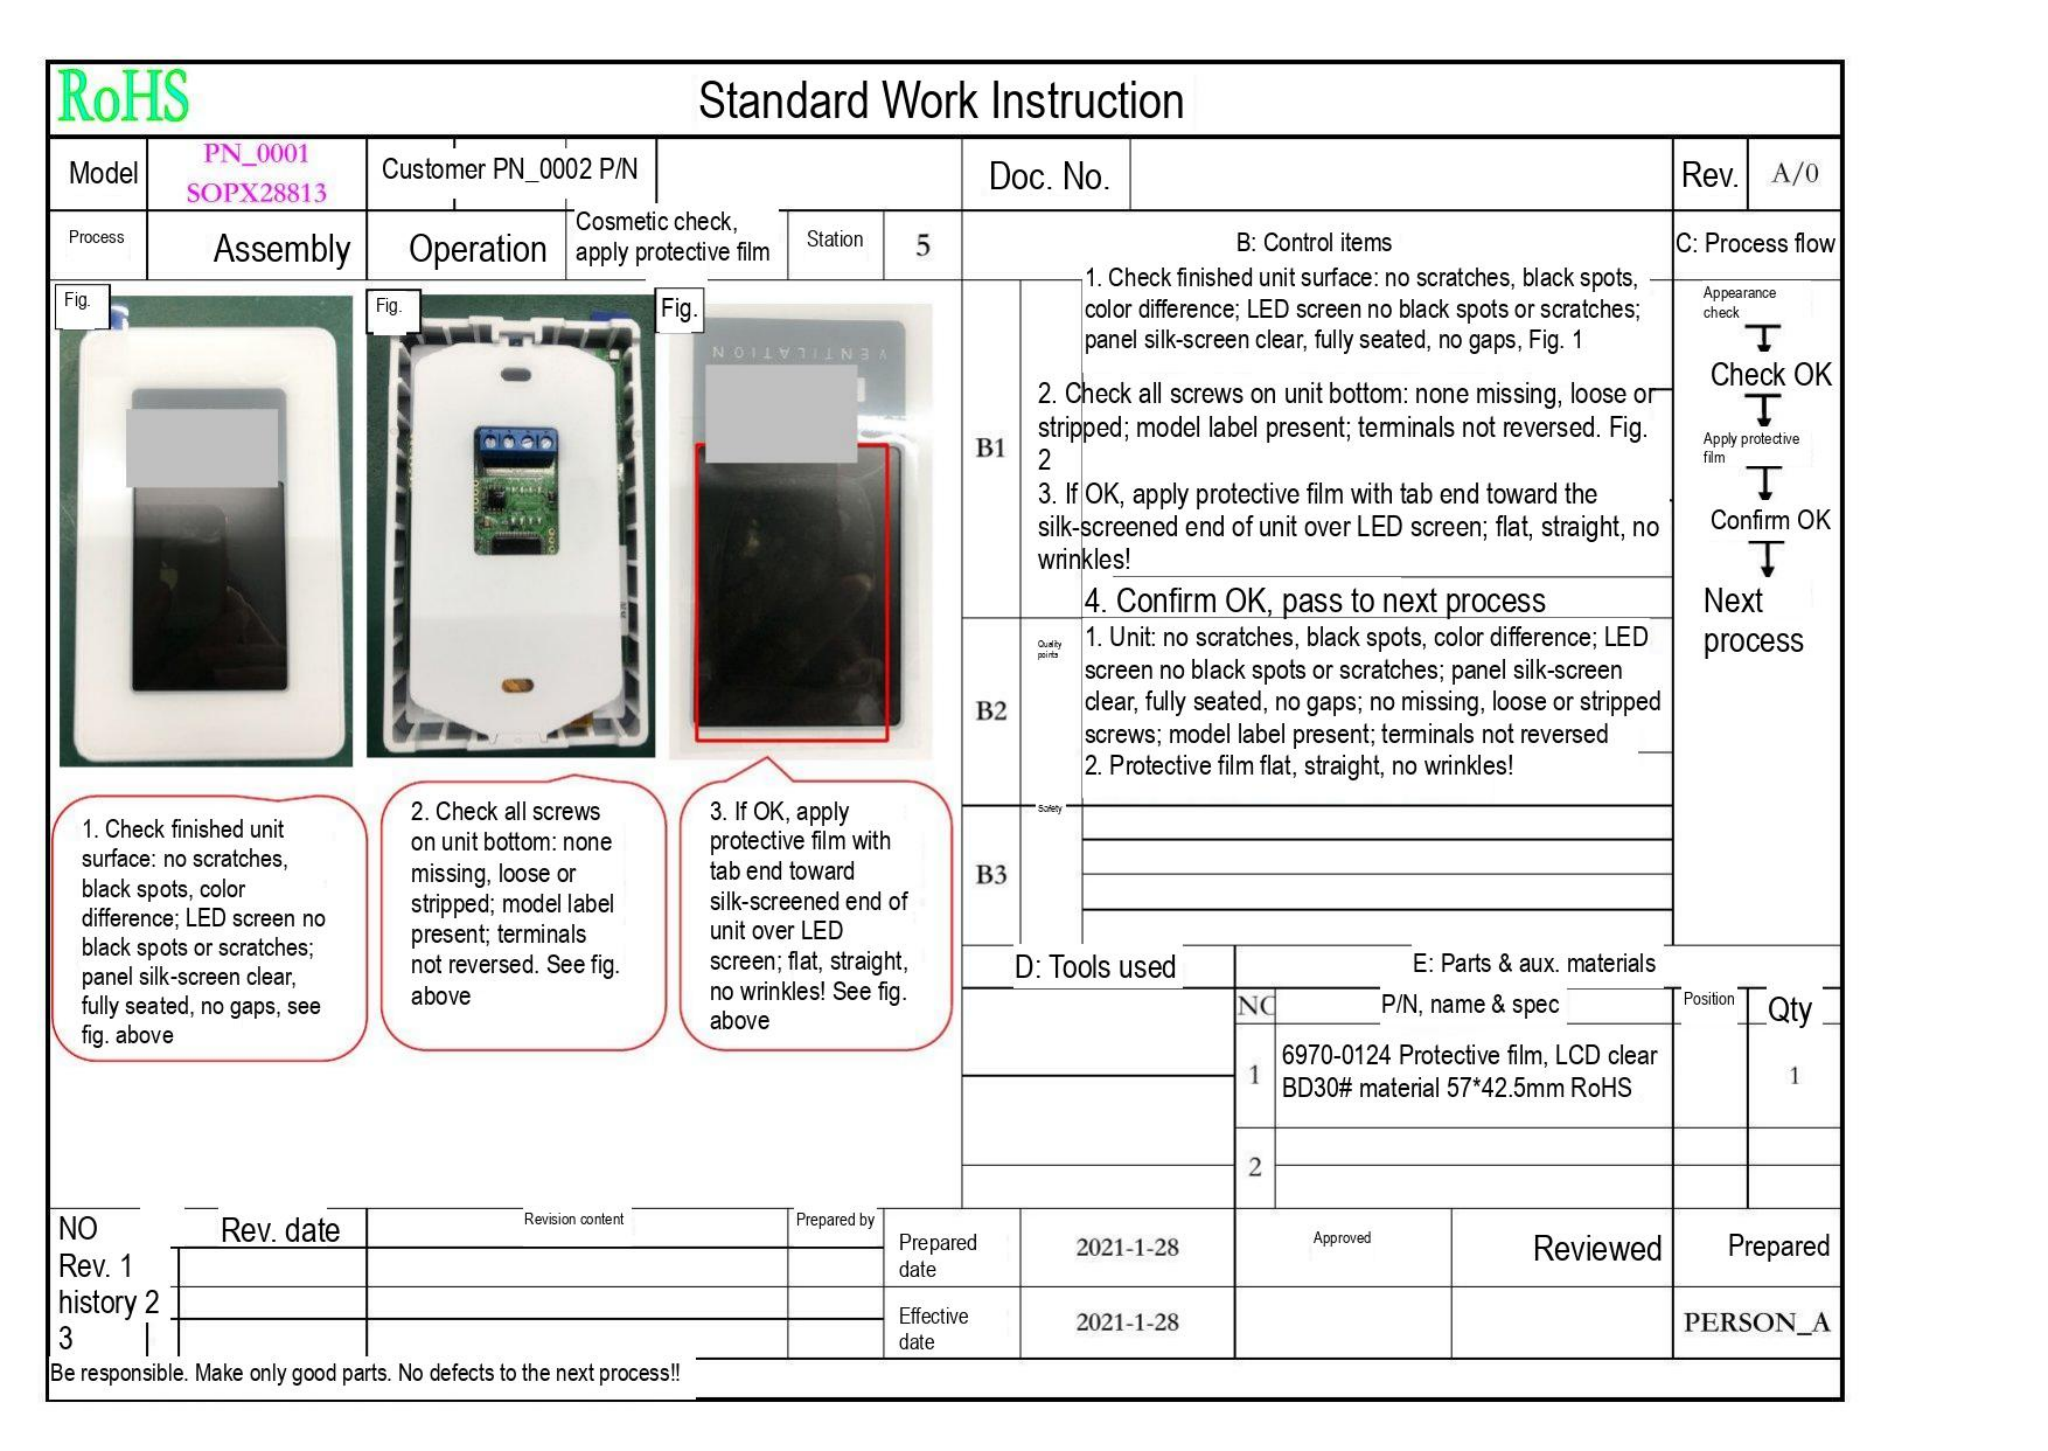RoHS

# Standard Work Instruction

| Model | PN_0001 SOPX28813 | Customer PN_0002 P/N | | Doc. No. | | Rev. | A/0 |
|---|---|---|---|---|---|---|---|
| Process | Assembly | Operation | Cosmetic check, apply protective film | Station | 5 | | |

Fig.

Fig.

Fig.

VENTILATION

1. Check finished unit surface: no scratches, black spots, color difference; LED screen no black spots or scratches; panel silk-screen clear, fully seated, no gaps, see fig. above

2. Check all screws on unit bottom: none missing, loose or stripped; model label present; terminals not reversed. See fig. above

3. If OK, apply protective film with tab end toward silk-screened end of unit over LED screen; flat, straight, no wrinkles! See fig. above

B: Control items

| | | |
|---|---|---|
| B1 | | 1. Check finished unit surface: no scratches, black spots, color difference; LED screen no black spots or scratches; panel silk-screen clear, fully seated, no gaps, Fig. 1<br>2. Check all screws on unit bottom: none missing, loose or stripped; model label present; terminals not reversed. Fig. 2<br>3. If OK, apply protective film with tab end toward the silk-screened end of unit over LED screen; flat, straight, no wrinkles!<br>4. Confirm OK, pass to next process |
| B2 | Quality points | 1. Unit: no scratches, black spots, color difference; LED screen no black spots or scratches; panel silk-screen clear, fully seated, no gaps; no missing, loose or stripped screws; model label present; terminals not reversed<br>2. Protective film flat, straight, no wrinkles! |
| B3 | Safety | |

C: Process flow

Appearance check
↓
Check OK
↓
Apply protective film
↓
Confirm OK
↓
Next process

D: Tools used

E: Parts & aux. materials

| NO | P/N, name & spec | Position | Qty |
|---|---|---|---|
| 1 | 6970-0124 Protective film, LCD clear BD30# material 57*42.5mm RoHS | | 1 |
| 2 | | | |

| NO | Rev. date | Revision content | Prepared by |
|---|---|---|---|
| Rev. 1 | | | |
| history 2 | | | |
| 3 | | | |

| | | Approved | Reviewed | Prepared |
|---|---|---|---|---|
| Prepared date | 2021-1-28 | | | |
| Effective date | 2021-1-28 | | | PERSON_A |

Be responsible. Make only good parts. No defects to the next process!!
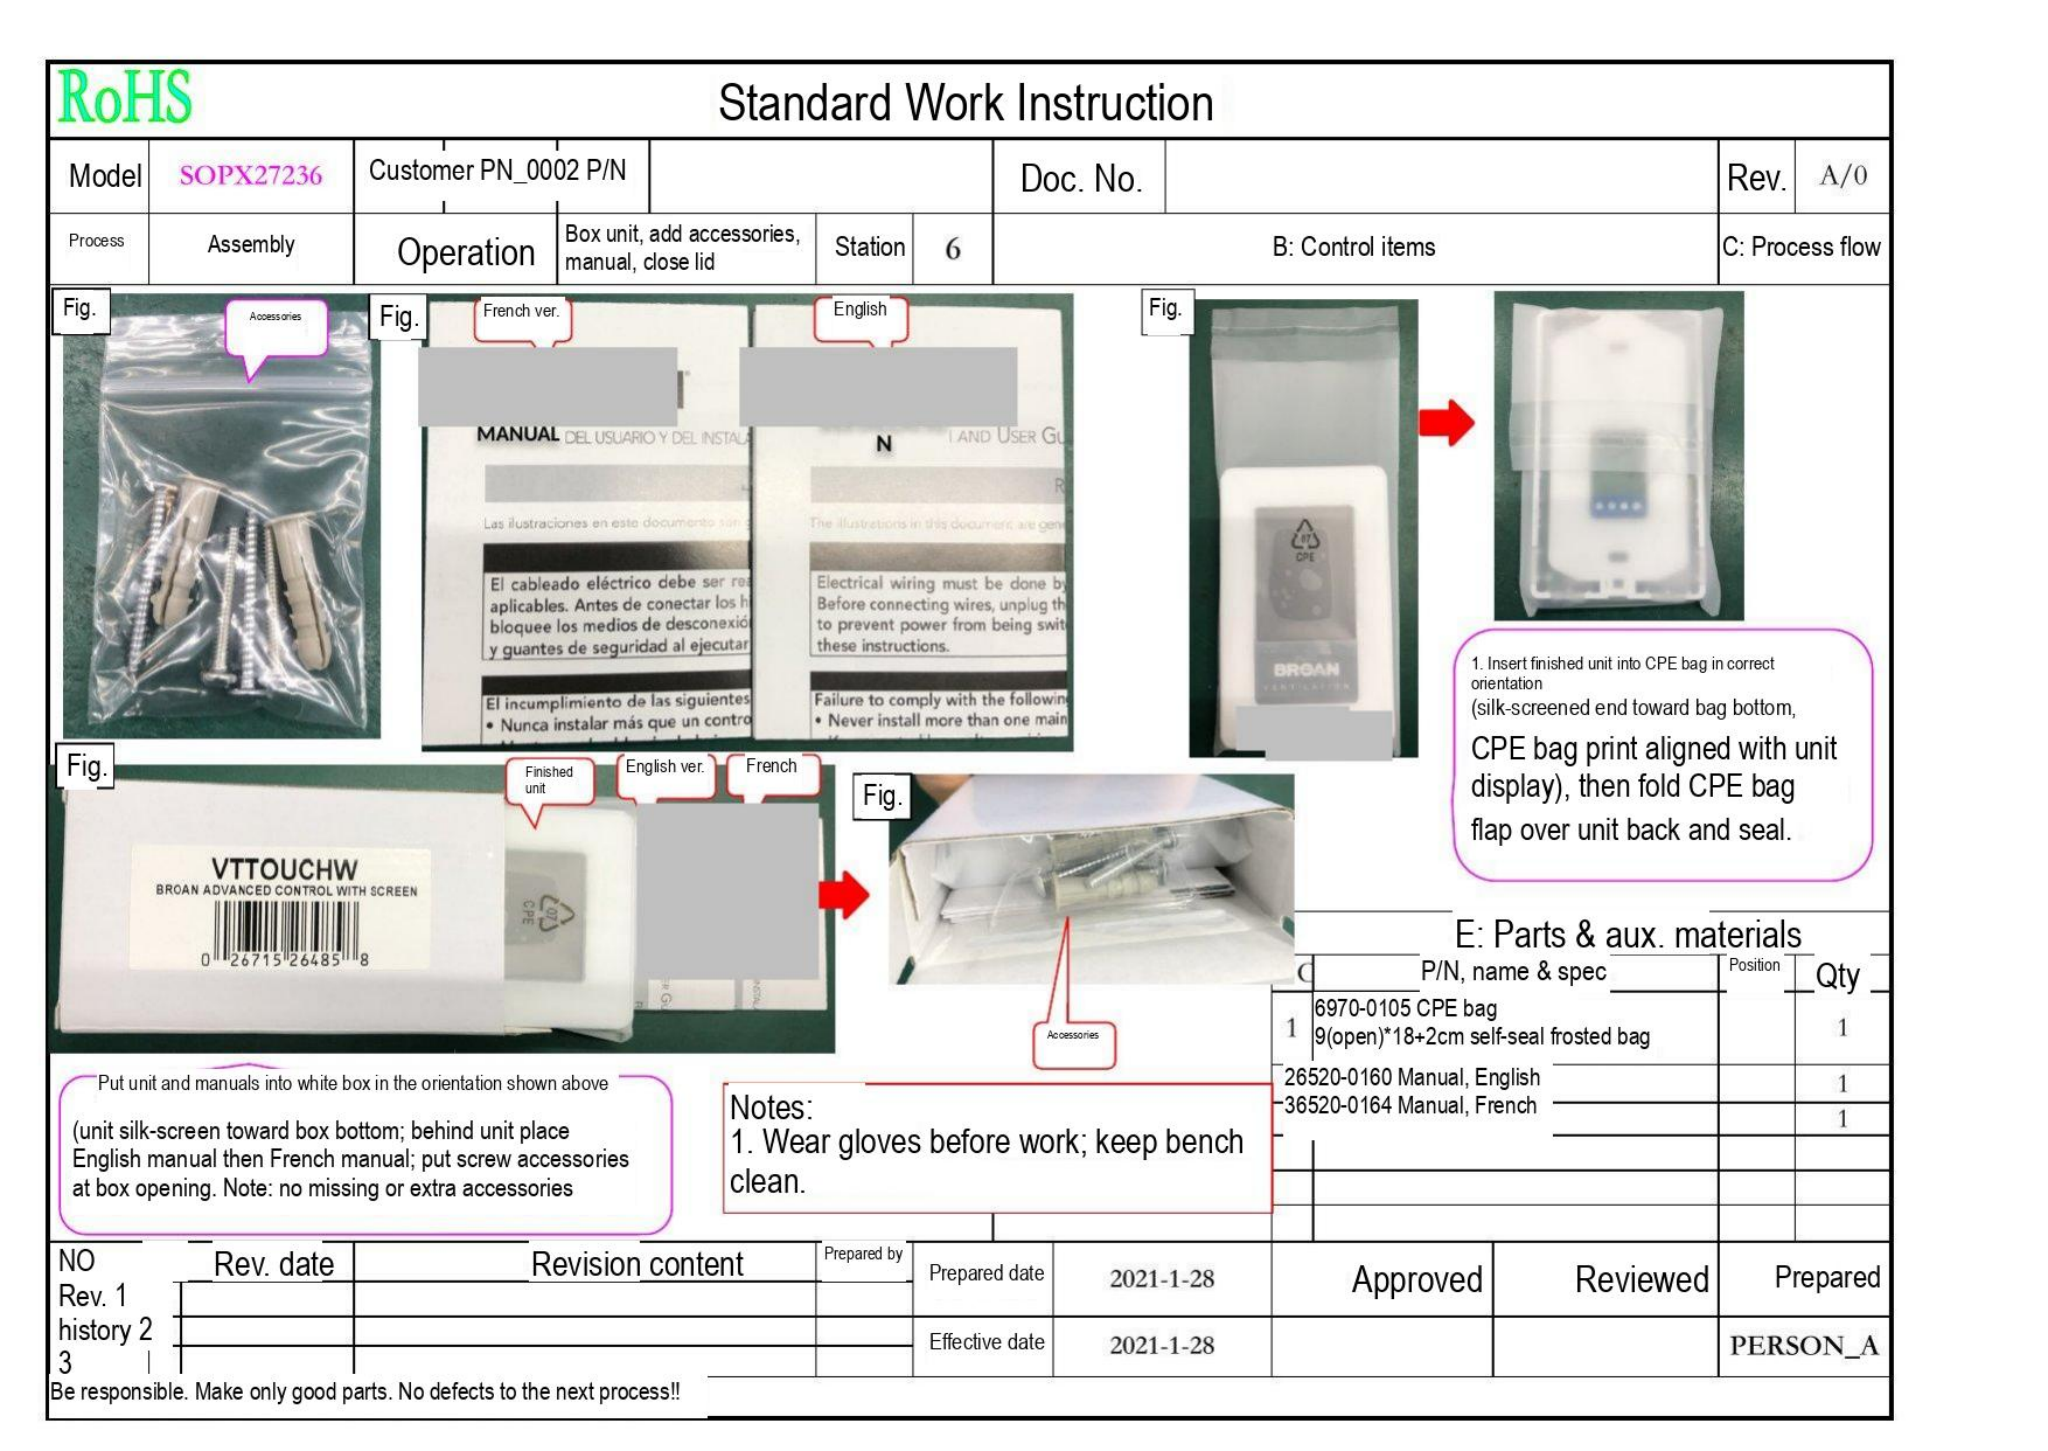RoHS

Standard Work Instruction

| Model | SOPX27236 | Customer PN_0002 P/N | | Doc. No. | | Rev. | A/0 |
|---|---|---|---|---|---|---|---|
| Process | Assembly | Operation | Box unit, add accessories, manual, close lid | Station | 6 | B: Control items | C: Process flow |

Fig.

Accessories

Fig.

French ver.

English

MANUAL DEL USUARIO Y DEL INSTALA

N

AND USER GU

Las ilustraciones en este documento son

The illustrations in this document are gen

El cableado eléctrico debe ser re
aplicables. Antes de conectar los h
bloquee los medios de desconexió
y guantes de seguridad al ejecutar

Electrical wiring must be done by
Before connecting wires, unplug th
to prevent power from being swit
these instructions.

El incumplimiento de las siguientes
• Nunca instalar más que un contro

Failure to comply with the followin
• Never install more than one main

Fig.

CPE

BROAN

1. Insert finished unit into CPE bag in correct orientation
(silk-screened end toward bag bottom,
CPE bag print aligned with unit display), then fold CPE bag flap over unit back and seal.

Fig.

Finished unit

English ver.

French

VTTOUCHW
BROAN ADVANCED CONTROL WITH SCREEN
0 26715 26485 8

CPE

Fig.

Accessories

Put unit and manuals into white box in the orientation shown above
(unit silk-screen toward box bottom; behind unit place English manual then French manual; put screw accessories at box opening. Note: no missing or extra accessories

Notes:
1. Wear gloves before work; keep bench clean.

E: Parts & aux. materials

| | P/N, name & spec | Position | Qty |
|---|---|---|---|
| 1 | 6970-0105 CPE bag<br>9(open)*18+2cm self-seal frosted bag | | 1 |
| | 26520-0160 Manual, English | | 1 |
| | 36520-0164 Manual, French | | 1 |
| | | | |
| | | | |
| | | | |

| NO | Rev. date | Revision content | Prepared by | Prepared date | 2021-1-28 | Approved | Reviewed | Prepared |
|---|---|---|---|---|---|---|---|---|
| Rev. 1 | | | | | | | | |
| history 2 | | | | Effective date | 2021-1-28 | | | PERSON_A |
| 3 | | | | | | | | |

Be responsible. Make only good parts. No defects to the next process!!
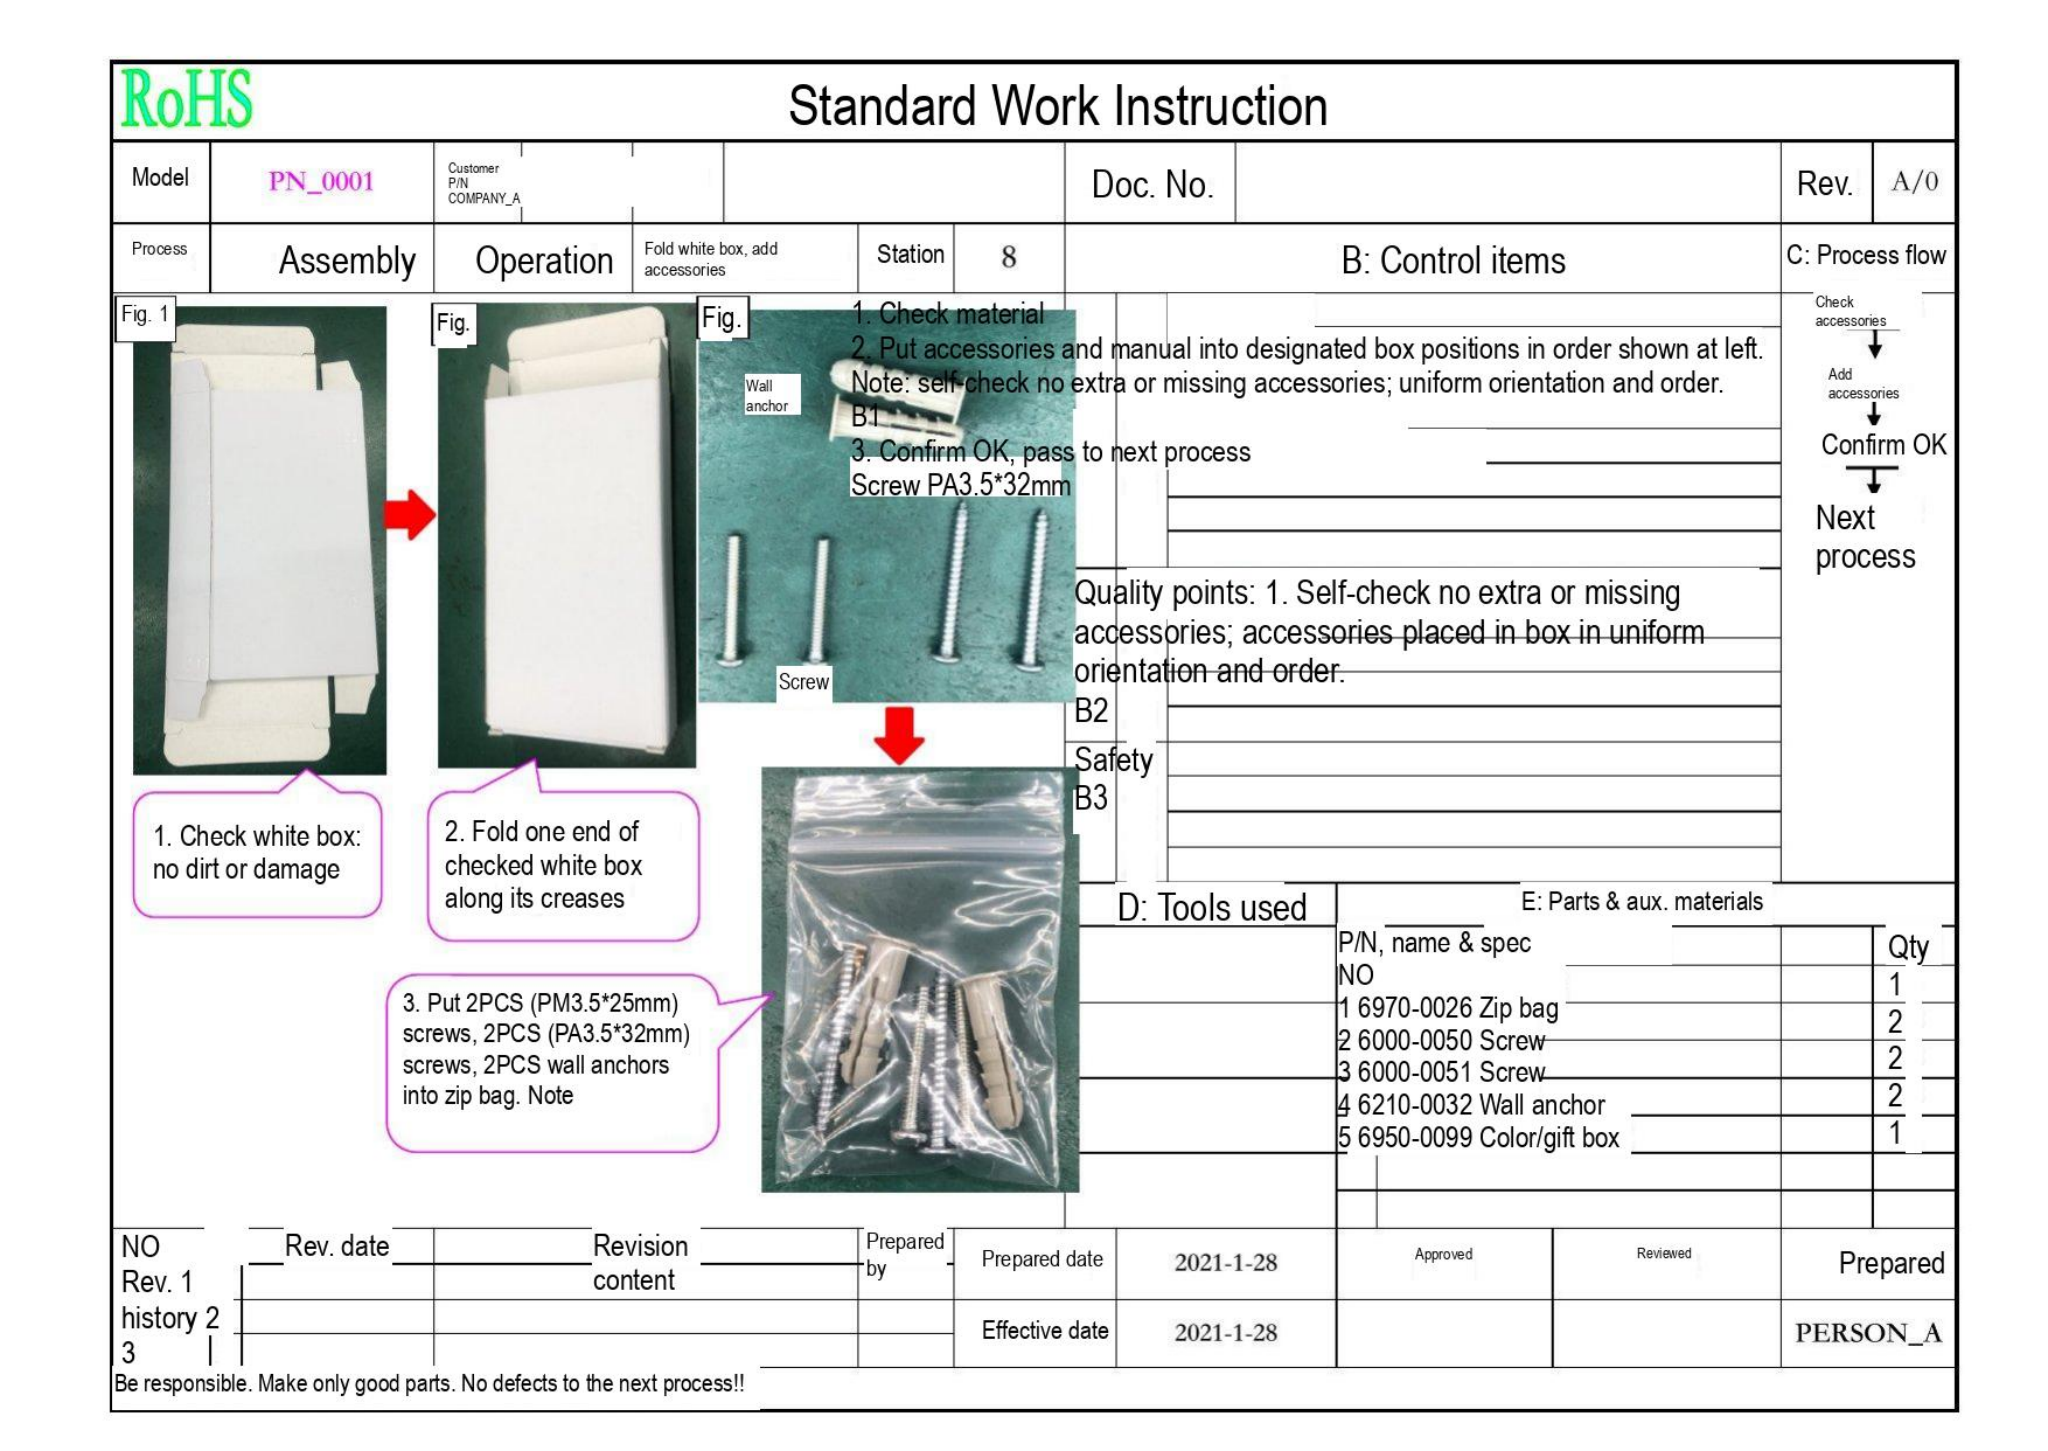RoHS

Standard Work Instruction

| Model | PN_0001 | Customer P/N COMPANY_A | | Doc. No. | | Rev. | A/0 |
|---|---|---|---|---|---|---|---|
| Process | Assembly | Operation | Fold white box, add accessories | Station | 8 | | |

Fig. 1

Fig.

Fig.

Wall anchor

Screw

1. Check white box: no dirt or damage

2. Fold one end of checked white box along its creases

3. Put 2PCS (PM3.5*25mm) screws, 2PCS (PA3.5*32mm) screws, 2PCS wall anchors into zip bag. Note

B: Control items

1. Check material
2. Put accessories and manual into designated box positions in order shown at left.
Note: self-check no extra or missing accessories; uniform orientation and order.
B1
3. Confirm OK, pass to next process
Screw PA3.5*32mm

Quality points: 1. Self-check no extra or missing accessories; accessories placed in box in uniform orientation and order.
B2
Safety
B3

C: Process flow

Check accessories
Add accessories
Confirm OK
Next process

D: Tools used

E: Parts & aux. materials

| NO | P/N, name & spec | Qty |
|---|---|---|
| 1 | 6970-0026 Zip bag | 1 |
| 2 | 6000-0050 Screw | 2 |
| 3 | 6000-0051 Screw | 2 |
| 4 | 6210-0032 Wall anchor | 2 |
| 5 | 6950-0099 Color/gift box | 1 |

| NO | Rev. date | Revision content | Prepared by | Prepared date | 2021-1-28 | Approved | Reviewed | Prepared |
|---|---|---|---|---|---|---|---|---|
| Rev. 1 | | | | | | | | |
| history 2 | | | | Effective date | 2021-1-28 | | | PERSON_A |
| 3 | | | | | | | | |

Be responsible. Make only good parts. No defects to the next process!!